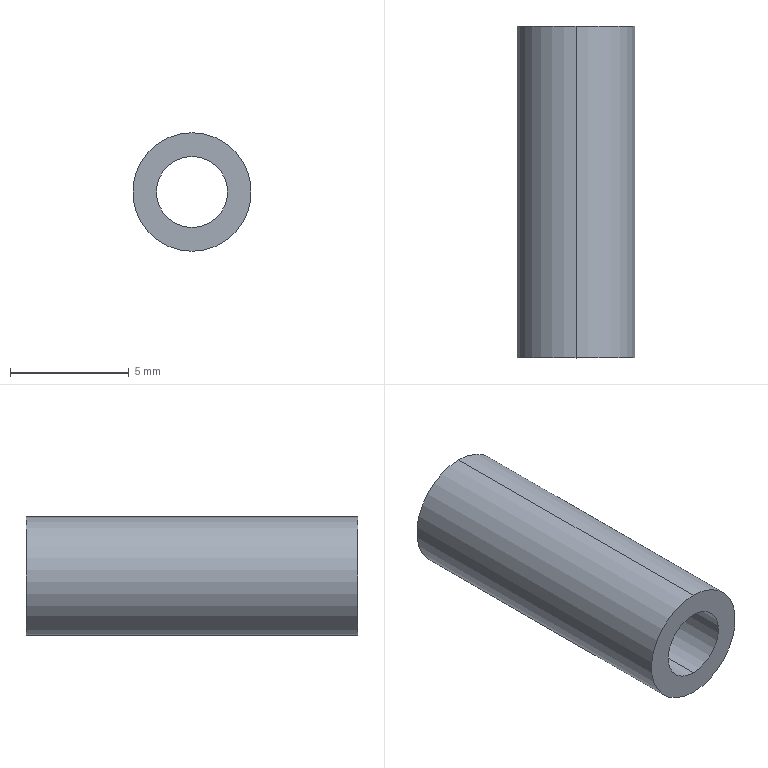Part | SolidWorks | features Extrusion 1 | 1 solid | 6 faces | box 5 x 14 x 5 mm | volume 175.929 mm3 | cylinder 4 | plane 2 | commonest cylinder face diameters 3 x2 5 x2
STEP:
#1=CARTESIAN_POINT('',(0.,14.,-1.5));
#2=VERTEX_POINT('',#1);
#3=CARTESIAN_POINT('',(0.,14.,1.5));
#4=VERTEX_POINT('',#3);
#5=CARTESIAN_POINT('',(0.,14.,0.));
#6=DIRECTION('',(0.,1.,0.));
#7=DIRECTION('',(0.,0.,1.));
#8=AXIS2_PLACEMENT_3D('',#5,#6,#7);
#9=CIRCLE('',#8,1.5);
#10=EDGE_CURVE('',#2,#4,#9,.T.);
#11=ORIENTED_EDGE('',*,*,#10,.T.);
#12=CARTESIAN_POINT('',(0.,0.,1.5));
#13=VERTEX_POINT('',#12);
#14=CARTESIAN_POINT('',(0.,14.,1.5));
#15=DIRECTION('',(0.,-1.,0.));
#16=VECTOR('',#15,1000.);
#17=LINE('',#14,#16);
#18=EDGE_CURVE('',#4,#13,#17,.T.);
#19=ORIENTED_EDGE('',*,*,#18,.T.);
#20=CARTESIAN_POINT('',(0.,0.,-1.5));
#21=VERTEX_POINT('',#20);
#22=CARTESIAN_POINT('',(0.,0.,0.));
#23=DIRECTION('',(0.,1.,0.));
#24=DIRECTION('',(0.,0.,1.));
#25=AXIS2_PLACEMENT_3D('',#22,#23,#24);
#26=CIRCLE('',#25,1.5);
#27=EDGE_CURVE('',#21,#13,#26,.T.);
#28=ORIENTED_EDGE('',*,*,#27,.F.);
#29=CARTESIAN_POINT('',(0.,14.,-1.5));
#30=DIRECTION('',(0.,-1.,0.));
#31=VECTOR('',#30,1000.);
#32=LINE('',#29,#31);
#33=EDGE_CURVE('',#2,#21,#32,.T.);
#34=ORIENTED_EDGE('',*,*,#33,.F.);
#35=EDGE_LOOP('',(#11,#19,#28,#34));
#36=FACE_OUTER_BOUND('',#35,.T.);
#37=CARTESIAN_POINT('',(0.,14.,0.));
#38=DIRECTION('',(0.,-1.,0.));
#39=DIRECTION('',(0.,0.,-1.));
#40=AXIS2_PLACEMENT_3D('',#37,#38,#39);
#41=CYLINDRICAL_SURFACE('',#40,1.5);
#42=ADVANCED_FACE('',(#36),#41,.F.);
#43=CARTESIAN_POINT('',(0.,14.,2.5));
#44=VERTEX_POINT('',#43);
#45=CARTESIAN_POINT('',(0.,14.,-2.5));
#46=VERTEX_POINT('',#45);
#47=CARTESIAN_POINT('',(0.,14.,0.));
#48=DIRECTION('',(0.,1.,0.));
#49=DIRECTION('',(0.,0.,1.));
#50=AXIS2_PLACEMENT_3D('',#47,#48,#49);
#51=CIRCLE('',#50,2.5);
#52=EDGE_CURVE('',#44,#46,#51,.T.);
#53=ORIENTED_EDGE('',*,*,#52,.F.);
#54=CARTESIAN_POINT('',(0.,0.,2.5));
#55=VERTEX_POINT('',#54);
#56=CARTESIAN_POINT('',(0.,14.,2.5));
#57=DIRECTION('',(0.,-1.,0.));
#58=VECTOR('',#57,1000.);
#59=LINE('',#56,#58);
#60=EDGE_CURVE('',#44,#55,#59,.T.);
#61=ORIENTED_EDGE('',*,*,#60,.T.);
#62=CARTESIAN_POINT('',(0.,0.,-2.5));
#63=VERTEX_POINT('',#62);
#64=CARTESIAN_POINT('',(0.,0.,0.));
#65=DIRECTION('',(0.,1.,0.));
#66=DIRECTION('',(0.,0.,1.));
#67=AXIS2_PLACEMENT_3D('',#64,#65,#66);
#68=CIRCLE('',#67,2.5);
#69=EDGE_CURVE('',#55,#63,#68,.T.);
#70=ORIENTED_EDGE('',*,*,#69,.T.);
#71=CARTESIAN_POINT('',(0.,14.,-2.5));
#72=DIRECTION('',(0.,-1.,0.));
#73=VECTOR('',#72,1000.);
#74=LINE('',#71,#73);
#75=EDGE_CURVE('',#46,#63,#74,.T.);
#76=ORIENTED_EDGE('',*,*,#75,.F.);
#77=EDGE_LOOP('',(#53,#61,#70,#76));
#78=FACE_OUTER_BOUND('',#77,.T.);
#79=CARTESIAN_POINT('',(0.,14.,0.));
#80=DIRECTION('',(0.,-1.,0.));
#81=DIRECTION('',(0.,0.,-1.));
#82=AXIS2_PLACEMENT_3D('',#79,#80,#81);
#83=CYLINDRICAL_SURFACE('',#82,2.5);
#84=ADVANCED_FACE('',(#78),#83,.T.);
#85=CARTESIAN_POINT('',(0.,14.,0.));
#86=DIRECTION('',(0.,1.,0.));
#87=DIRECTION('',(0.,0.,1.));
#88=AXIS2_PLACEMENT_3D('',#85,#86,#87);
#89=CIRCLE('',#88,2.5);
#90=EDGE_CURVE('',#46,#44,#89,.T.);
#91=ORIENTED_EDGE('',*,*,#90,.T.);
#92=ORIENTED_EDGE('',*,*,#52,.T.);
#93=EDGE_LOOP('',(#91,#92));
#94=FACE_OUTER_BOUND('',#93,.T.);
#95=ORIENTED_EDGE('',*,*,#10,.F.);
#96=CARTESIAN_POINT('',(0.,14.,0.));
#97=DIRECTION('',(0.,1.,0.));
#98=DIRECTION('',(0.,0.,1.));
#99=AXIS2_PLACEMENT_3D('',#96,#97,#98);
#100=CIRCLE('',#99,1.5);
#101=EDGE_CURVE('',#4,#2,#100,.T.);
#102=ORIENTED_EDGE('',*,*,#101,.F.);
#103=EDGE_LOOP('',(#95,#102));
#104=FACE_BOUND('',#103,.T.);
#105=CARTESIAN_POINT('',(0.,14.,0.));
#106=DIRECTION('',(0.,1.,0.));
#107=DIRECTION('',(0.,0.,1.));
#108=AXIS2_PLACEMENT_3D('',#105,#106,#107);
#109=PLANE('',#108);
#110=ADVANCED_FACE('',(#94,#104),#109,.T.);
#111=CARTESIAN_POINT('',(0.,0.,0.));
#112=DIRECTION('',(0.,1.,0.));
#113=DIRECTION('',(0.,0.,1.));
#114=AXIS2_PLACEMENT_3D('',#111,#112,#113);
#115=CIRCLE('',#114,2.5);
#116=EDGE_CURVE('',#63,#55,#115,.T.);
#117=ORIENTED_EDGE('',*,*,#116,.F.);
#118=ORIENTED_EDGE('',*,*,#69,.F.);
#119=EDGE_LOOP('',(#117,#118));
#120=FACE_OUTER_BOUND('',#119,.T.);
#121=ORIENTED_EDGE('',*,*,#27,.T.);
#122=CARTESIAN_POINT('',(0.,0.,0.));
#123=DIRECTION('',(0.,1.,0.));
#124=DIRECTION('',(0.,0.,1.));
#125=AXIS2_PLACEMENT_3D('',#122,#123,#124);
#126=CIRCLE('',#125,1.5);
#127=EDGE_CURVE('',#13,#21,#126,.T.);
#128=ORIENTED_EDGE('',*,*,#127,.T.);
#129=EDGE_LOOP('',(#121,#128));
#130=FACE_BOUND('',#129,.T.);
#131=CARTESIAN_POINT('',(0.,0.,0.));
#132=DIRECTION('',(0.,1.,0.));
#133=DIRECTION('',(0.,0.,1.));
#134=AXIS2_PLACEMENT_3D('',#131,#132,#133);
#135=PLANE('',#134);
#136=ADVANCED_FACE('',(#120,#130),#135,.F.);
#137=ORIENTED_EDGE('',*,*,#60,.F.);
#138=ORIENTED_EDGE('',*,*,#90,.F.);
#139=ORIENTED_EDGE('',*,*,#75,.T.);
#140=ORIENTED_EDGE('',*,*,#116,.T.);
#141=EDGE_LOOP('',(#137,#138,#139,#140));
#142=FACE_OUTER_BOUND('',#141,.T.);
#143=CARTESIAN_POINT('',(0.,14.,0.));
#144=DIRECTION('',(0.,-1.,0.));
#145=DIRECTION('',(0.,0.,-1.));
#146=AXIS2_PLACEMENT_3D('',#143,#144,#145);
#147=CYLINDRICAL_SURFACE('',#146,2.5);
#148=ADVANCED_FACE('',(#142),#147,.T.);
#149=ORIENTED_EDGE('',*,*,#18,.F.);
#150=ORIENTED_EDGE('',*,*,#101,.T.);
#151=ORIENTED_EDGE('',*,*,#33,.T.);
#152=ORIENTED_EDGE('',*,*,#127,.F.);
#153=EDGE_LOOP('',(#149,#150,#151,#152));
#154=FACE_OUTER_BOUND('',#153,.T.);
#155=CARTESIAN_POINT('',(0.,14.,0.));
#156=DIRECTION('',(0.,-1.,0.));
#157=DIRECTION('',(0.,0.,-1.));
#158=AXIS2_PLACEMENT_3D('',#155,#156,#157);
#159=CYLINDRICAL_SURFACE('',#158,1.5);
#160=ADVANCED_FACE('',(#154),#159,.F.);
#161=CLOSED_SHELL('',(#42,#84,#110,#136,#148,#160));
#162=MANIFOLD_SOLID_BREP('',#161);
#163=CARTESIAN_POINT('',(0.,0.,0.));
#164=DIRECTION('',(0.,0.,1.));
#165=DIRECTION('',(1.,0.,0.));
#166=AXIS2_PLACEMENT_3D('',#163,#164,#165);
#167=(LENGTH_UNIT()NAMED_UNIT(*)SI_UNIT(.MILLI.,.METRE.));
#168=UNCERTAINTY_MEASURE_WITH_UNIT(LENGTH_MEASURE(0.00001),#167,'','');
#169=(NAMED_UNIT(*)PLANE_ANGLE_UNIT()SI_UNIT($,.RADIAN.));
#170=(NAMED_UNIT(*)SI_UNIT($,.STERADIAN.)SOLID_ANGLE_UNIT());
#171=(GEOMETRIC_REPRESENTATION_CONTEXT(3)GLOBAL_UNCERTAINTY_ASSIGNED_CONTEXT((#168))GLOBAL_UNIT_ASSIGNED_CONTEXT((#167,#169,#170))REPRESENTATION_CONTEXT('',''));
#172=ADVANCED_BREP_SHAPE_REPRESENTATION('',(#162,#166),#171);